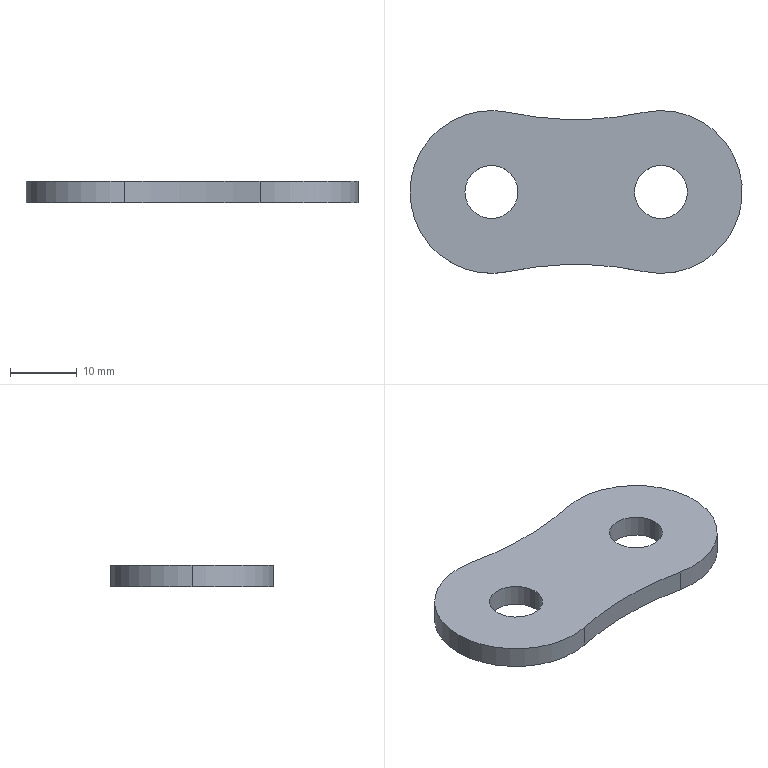Part | STEP file | Outer chain link | 1 solid | 11 faces | box 49.79 x 24.39 x 3.25 mm | volume 3077 mm3 | cylinder 9 | plane 2 | commonest cylinder face diameters 7.94 x4 24.39 x3 97.627 x2
STEP:
#1=CARTESIAN_POINT('',(0.,0.,0.));
#2=DIRECTION('',(0.,0.,1.));
#3=DIRECTION('',(1.,0.,0.));
#4=AXIS2_PLACEMENT_3D('',#1,#2,#3);
#5=CARTESIAN_POINT('',(16.67,0.,0.));
#6=VERTEX_POINT('',#5);
#7=CARTESIAN_POINT('',(16.67,0.,3.25));
#8=VERTEX_POINT('',#7);
#9=CARTESIAN_POINT('',(16.67,0.,0.));
#10=DIRECTION('',(0.,0.,1.));
#11=VECTOR('',#10,1.);
#12=LINE('',#9,#11);
#13=CARTESIAN_POINT('',(12.7,0.,0.));
#14=DIRECTION('',(0.,0.,1.));
#15=DIRECTION('',(1.,0.,0.));
#16=AXIS2_PLACEMENT_3D('',#13,#14,#15);
#17=CYLINDRICAL_SURFACE('',#16,3.97);
#18=CARTESIAN_POINT('',(6.283,0.));
#19=DIRECTION('',(0.,1.));
#20=VECTOR('',#19,1.);
#21=LINE('',#18,#20);
#22=(GEOMETRIC_REPRESENTATION_CONTEXT(2)PARAMETRIC_REPRESENTATION_CONTEXT()REPRESENTATION_CONTEXT('',''));
#23=DEFINITIONAL_REPRESENTATION('',(#21),#22);
#24=PCURVE('',#17,#23);
#25=CARTESIAN_POINT('',(12.7,0.,0.));
#26=DIRECTION('',(0.,0.,1.));
#27=DIRECTION('',(1.,0.,0.));
#28=AXIS2_PLACEMENT_3D('',#25,#26,#27);
#29=CYLINDRICAL_SURFACE('',#28,3.97);
#30=CARTESIAN_POINT('',(0.,0.));
#31=DIRECTION('',(0.,1.));
#32=VECTOR('',#31,1.);
#33=LINE('',#30,#32);
#34=(GEOMETRIC_REPRESENTATION_CONTEXT(2)PARAMETRIC_REPRESENTATION_CONTEXT()REPRESENTATION_CONTEXT('',''));
#35=DEFINITIONAL_REPRESENTATION('',(#33),#34);
#36=PCURVE('',#29,#35);
#37=SURFACE_CURVE('',#12,(#24,#36),.PCURVE_S1.);
#38=EDGE_CURVE('',#6,#8,#37,.T.);
#39=ORIENTED_EDGE('',*,*,#38,.T.);
#40=CARTESIAN_POINT('',(8.73,0.,3.25));
#41=VERTEX_POINT('',#40);
#42=CARTESIAN_POINT('',(12.7,0.,3.25));
#43=DIRECTION('',(0.,0.,1.));
#44=DIRECTION('',(1.,0.,0.));
#45=AXIS2_PLACEMENT_3D('',#42,#43,#44);
#46=CIRCLE('',#45,3.97);
#47=CARTESIAN_POINT('',(0.,3.25));
#48=DIRECTION('',(1.,0.));
#49=VECTOR('',#48,1.);
#50=LINE('',#47,#49);
#51=(GEOMETRIC_REPRESENTATION_CONTEXT(2)PARAMETRIC_REPRESENTATION_CONTEXT()REPRESENTATION_CONTEXT('',''));
#52=DEFINITIONAL_REPRESENTATION('',(#50),#51);
#53=PCURVE('',#17,#52);
#54=CARTESIAN_POINT('',(-6.35,-29.836,3.25));
#55=DIRECTION('',(0.,0.,1.));
#56=DIRECTION('',(1.,0.,0.));
#57=AXIS2_PLACEMENT_3D('',#54,#55,#56);
#58=PLANE('',#57);
#59=CARTESIAN_POINT('',(19.05,29.836));
#60=DIRECTION('',(1.,0.));
#61=AXIS2_PLACEMENT_2D('',#59,#60);
#62=CIRCLE('',#61,3.97);
#63=(GEOMETRIC_REPRESENTATION_CONTEXT(2)PARAMETRIC_REPRESENTATION_CONTEXT()REPRESENTATION_CONTEXT('',''));
#64=DEFINITIONAL_REPRESENTATION('',(#62),#63);
#65=PCURVE('',#58,#64);
#66=SURFACE_CURVE('',#46,(#53,#65),.PCURVE_S1.);
#67=EDGE_CURVE('',#41,#8,#66,.T.);
#68=ORIENTED_EDGE('',*,*,#67,.F.);
#69=CARTESIAN_POINT('',(8.73,0.,0.));
#70=VERTEX_POINT('',#69);
#71=CARTESIAN_POINT('',(8.73,0.,0.));
#72=DIRECTION('',(0.,0.,1.));
#73=VECTOR('',#72,1.);
#74=LINE('',#71,#73);
#75=CARTESIAN_POINT('',(3.142,0.));
#76=DIRECTION('',(0.,1.));
#77=VECTOR('',#76,1.);
#78=LINE('',#75,#77);
#79=(GEOMETRIC_REPRESENTATION_CONTEXT(2)PARAMETRIC_REPRESENTATION_CONTEXT()REPRESENTATION_CONTEXT('',''));
#80=DEFINITIONAL_REPRESENTATION('',(#78),#79);
#81=PCURVE('',#17,#80);
#82=CARTESIAN_POINT('',(3.142,0.));
#83=DIRECTION('',(0.,1.));
#84=VECTOR('',#83,1.);
#85=LINE('',#82,#84);
#86=(GEOMETRIC_REPRESENTATION_CONTEXT(2)PARAMETRIC_REPRESENTATION_CONTEXT()REPRESENTATION_CONTEXT('',''));
#87=DEFINITIONAL_REPRESENTATION('',(#85),#86);
#88=PCURVE('',#29,#87);
#89=SURFACE_CURVE('',#74,(#81,#88),.PCURVE_S1.);
#90=EDGE_CURVE('',#70,#41,#89,.T.);
#91=ORIENTED_EDGE('',*,*,#90,.F.);
#92=CARTESIAN_POINT('',(12.7,0.,0.));
#93=DIRECTION('',(0.,0.,1.));
#94=DIRECTION('',(1.,0.,0.));
#95=AXIS2_PLACEMENT_3D('',#92,#93,#94);
#96=CIRCLE('',#95,3.97);
#97=CARTESIAN_POINT('',(0.,0.));
#98=DIRECTION('',(1.,0.));
#99=VECTOR('',#98,1.);
#100=LINE('',#97,#99);
#101=(GEOMETRIC_REPRESENTATION_CONTEXT(2)PARAMETRIC_REPRESENTATION_CONTEXT()REPRESENTATION_CONTEXT('',''));
#102=DEFINITIONAL_REPRESENTATION('',(#100),#101);
#103=PCURVE('',#17,#102);
#104=CARTESIAN_POINT('',(-6.35,-29.836,0.));
#105=DIRECTION('',(0.,0.,1.));
#106=DIRECTION('',(1.,0.,0.));
#107=AXIS2_PLACEMENT_3D('',#104,#105,#106);
#108=PLANE('',#107);
#109=CARTESIAN_POINT('',(19.05,29.836));
#110=DIRECTION('',(1.,0.));
#111=AXIS2_PLACEMENT_2D('',#109,#110);
#112=CIRCLE('',#111,3.97);
#113=(GEOMETRIC_REPRESENTATION_CONTEXT(2)PARAMETRIC_REPRESENTATION_CONTEXT()REPRESENTATION_CONTEXT('',''));
#114=DEFINITIONAL_REPRESENTATION('',(#112),#113);
#115=PCURVE('',#108,#114);
#116=SURFACE_CURVE('',#96,(#103,#115),.PCURVE_S1.);
#117=EDGE_CURVE('',#70,#6,#116,.T.);
#118=ORIENTED_EDGE('',*,*,#117,.T.);
#119=EDGE_LOOP('',(#39,#68,#91,#118));
#120=FACE_BOUND('',#119,.F.);
#121=ADVANCED_FACE('',(#120),#17,.F.);
#122=CARTESIAN_POINT('',(-8.73,0.,0.));
#123=VERTEX_POINT('',#122);
#124=CARTESIAN_POINT('',(-8.73,0.,3.25));
#125=VERTEX_POINT('',#124);
#126=CARTESIAN_POINT('',(-8.73,0.,0.));
#127=DIRECTION('',(0.,0.,1.));
#128=VECTOR('',#127,1.);
#129=LINE('',#126,#128);
#130=CARTESIAN_POINT('',(-12.7,0.,0.));
#131=DIRECTION('',(0.,0.,1.));
#132=DIRECTION('',(1.,0.,0.));
#133=AXIS2_PLACEMENT_3D('',#130,#131,#132);
#134=CYLINDRICAL_SURFACE('',#133,3.97);
#135=CARTESIAN_POINT('',(6.283,0.));
#136=DIRECTION('',(0.,1.));
#137=VECTOR('',#136,1.);
#138=LINE('',#135,#137);
#139=(GEOMETRIC_REPRESENTATION_CONTEXT(2)PARAMETRIC_REPRESENTATION_CONTEXT()REPRESENTATION_CONTEXT('',''));
#140=DEFINITIONAL_REPRESENTATION('',(#138),#139);
#141=PCURVE('',#134,#140);
#142=CARTESIAN_POINT('',(-12.7,0.,0.));
#143=DIRECTION('',(0.,0.,1.));
#144=DIRECTION('',(1.,0.,0.));
#145=AXIS2_PLACEMENT_3D('',#142,#143,#144);
#146=CYLINDRICAL_SURFACE('',#145,3.97);
#147=CARTESIAN_POINT('',(0.,0.));
#148=DIRECTION('',(0.,1.));
#149=VECTOR('',#148,1.);
#150=LINE('',#147,#149);
#151=(GEOMETRIC_REPRESENTATION_CONTEXT(2)PARAMETRIC_REPRESENTATION_CONTEXT()REPRESENTATION_CONTEXT('',''));
#152=DEFINITIONAL_REPRESENTATION('',(#150),#151);
#153=PCURVE('',#146,#152);
#154=SURFACE_CURVE('',#129,(#141,#153),.PCURVE_S1.);
#155=EDGE_CURVE('',#123,#125,#154,.T.);
#156=ORIENTED_EDGE('',*,*,#155,.T.);
#157=CARTESIAN_POINT('',(-16.67,0.,3.25));
#158=VERTEX_POINT('',#157);
#159=CARTESIAN_POINT('',(-12.7,0.,3.25));
#160=DIRECTION('',(0.,0.,1.));
#161=DIRECTION('',(1.,0.,0.));
#162=AXIS2_PLACEMENT_3D('',#159,#160,#161);
#163=CIRCLE('',#162,3.97);
#164=CARTESIAN_POINT('',(0.,3.25));
#165=DIRECTION('',(1.,0.));
#166=VECTOR('',#165,1.);
#167=LINE('',#164,#166);
#168=(GEOMETRIC_REPRESENTATION_CONTEXT(2)PARAMETRIC_REPRESENTATION_CONTEXT()REPRESENTATION_CONTEXT('',''));
#169=DEFINITIONAL_REPRESENTATION('',(#167),#168);
#170=PCURVE('',#134,#169);
#171=CARTESIAN_POINT('',(-6.35,29.836));
#172=DIRECTION('',(1.,0.));
#173=AXIS2_PLACEMENT_2D('',#171,#172);
#174=CIRCLE('',#173,3.97);
#175=(GEOMETRIC_REPRESENTATION_CONTEXT(2)PARAMETRIC_REPRESENTATION_CONTEXT()REPRESENTATION_CONTEXT('',''));
#176=DEFINITIONAL_REPRESENTATION('',(#174),#175);
#177=PCURVE('',#58,#176);
#178=SURFACE_CURVE('',#163,(#170,#177),.PCURVE_S1.);
#179=EDGE_CURVE('',#158,#125,#178,.T.);
#180=ORIENTED_EDGE('',*,*,#179,.F.);
#181=CARTESIAN_POINT('',(-16.67,0.,0.));
#182=VERTEX_POINT('',#181);
#183=CARTESIAN_POINT('',(-16.67,0.,0.));
#184=DIRECTION('',(0.,0.,1.));
#185=VECTOR('',#184,1.);
#186=LINE('',#183,#185);
#187=CARTESIAN_POINT('',(3.142,0.));
#188=DIRECTION('',(0.,1.));
#189=VECTOR('',#188,1.);
#190=LINE('',#187,#189);
#191=(GEOMETRIC_REPRESENTATION_CONTEXT(2)PARAMETRIC_REPRESENTATION_CONTEXT()REPRESENTATION_CONTEXT('',''));
#192=DEFINITIONAL_REPRESENTATION('',(#190),#191);
#193=PCURVE('',#134,#192);
#194=CARTESIAN_POINT('',(3.142,0.));
#195=DIRECTION('',(0.,1.));
#196=VECTOR('',#195,1.);
#197=LINE('',#194,#196);
#198=(GEOMETRIC_REPRESENTATION_CONTEXT(2)PARAMETRIC_REPRESENTATION_CONTEXT()REPRESENTATION_CONTEXT('',''));
#199=DEFINITIONAL_REPRESENTATION('',(#197),#198);
#200=PCURVE('',#146,#199);
#201=SURFACE_CURVE('',#186,(#193,#200),.PCURVE_S1.);
#202=EDGE_CURVE('',#182,#158,#201,.T.);
#203=ORIENTED_EDGE('',*,*,#202,.F.);
#204=CARTESIAN_POINT('',(-12.7,0.,0.));
#205=DIRECTION('',(0.,0.,1.));
#206=DIRECTION('',(1.,0.,0.));
#207=AXIS2_PLACEMENT_3D('',#204,#205,#206);
#208=CIRCLE('',#207,3.97);
#209=CARTESIAN_POINT('',(0.,0.));
#210=DIRECTION('',(1.,0.));
#211=VECTOR('',#210,1.);
#212=LINE('',#209,#211);
#213=(GEOMETRIC_REPRESENTATION_CONTEXT(2)PARAMETRIC_REPRESENTATION_CONTEXT()REPRESENTATION_CONTEXT('',''));
#214=DEFINITIONAL_REPRESENTATION('',(#212),#213);
#215=PCURVE('',#134,#214);
#216=CARTESIAN_POINT('',(-6.35,29.836));
#217=DIRECTION('',(1.,0.));
#218=AXIS2_PLACEMENT_2D('',#216,#217);
#219=CIRCLE('',#218,3.97);
#220=(GEOMETRIC_REPRESENTATION_CONTEXT(2)PARAMETRIC_REPRESENTATION_CONTEXT()REPRESENTATION_CONTEXT('',''));
#221=DEFINITIONAL_REPRESENTATION('',(#219),#220);
#222=PCURVE('',#108,#221);
#223=SURFACE_CURVE('',#208,(#215,#222),.PCURVE_S1.);
#224=EDGE_CURVE('',#182,#123,#223,.T.);
#225=ORIENTED_EDGE('',*,*,#224,.T.);
#226=EDGE_LOOP('',(#156,#180,#203,#225));
#227=FACE_BOUND('',#226,.F.);
#228=ADVANCED_FACE('',(#227),#134,.F.);
#229=CARTESIAN_POINT('',(-24.895,0.,3.25));
#230=VERTEX_POINT('',#229);
#231=CARTESIAN_POINT('',(-10.161,-11.928,3.25));
#232=VERTEX_POINT('',#231);
#233=CARTESIAN_POINT('',(-12.7,0.,3.25));
#234=DIRECTION('',(0.,0.,1.));
#235=DIRECTION('',(1.,0.,0.));
#236=AXIS2_PLACEMENT_3D('',#233,#234,#235);
#237=CIRCLE('',#236,12.195);
#238=CARTESIAN_POINT('',(-12.7,0.,3.25));
#239=DIRECTION('',(0.,0.,-1.));
#240=DIRECTION('',(-1.,0.,0.));
#241=AXIS2_PLACEMENT_3D('',#238,#239,#240);
#242=CYLINDRICAL_SURFACE('',#241,12.195);
#243=CARTESIAN_POINT('',(9.425,0.));
#244=DIRECTION('',(-1.,0.));
#245=VECTOR('',#244,1.);
#246=LINE('',#243,#245);
#247=(GEOMETRIC_REPRESENTATION_CONTEXT(2)PARAMETRIC_REPRESENTATION_CONTEXT()REPRESENTATION_CONTEXT('',''));
#248=DEFINITIONAL_REPRESENTATION('',(#246),#247);
#249=PCURVE('',#242,#248);
#250=CARTESIAN_POINT('',(-6.35,29.836));
#251=DIRECTION('',(1.,0.));
#252=AXIS2_PLACEMENT_2D('',#250,#251);
#253=CIRCLE('',#252,12.195);
#254=(GEOMETRIC_REPRESENTATION_CONTEXT(2)PARAMETRIC_REPRESENTATION_CONTEXT()REPRESENTATION_CONTEXT('',''));
#255=DEFINITIONAL_REPRESENTATION('',(#253),#254);
#256=PCURVE('',#58,#255);
#257=SURFACE_CURVE('',#237,(#249,#256),.PCURVE_S1.);
#258=EDGE_CURVE('',#230,#232,#257,.T.);
#259=ORIENTED_EDGE('',*,*,#258,.F.);
#260=CARTESIAN_POINT('',(-24.895,0.,0.));
#261=VERTEX_POINT('',#260);
#262=CARTESIAN_POINT('',(-24.895,0.,3.25));
#263=DIRECTION('',(0.,0.,-1.));
#264=VECTOR('',#263,1.);
#265=LINE('',#262,#264);
#266=CARTESIAN_POINT('',(6.283,0.));
#267=DIRECTION('',(0.,1.));
#268=VECTOR('',#267,1.);
#269=LINE('',#266,#268);
#270=(GEOMETRIC_REPRESENTATION_CONTEXT(2)PARAMETRIC_REPRESENTATION_CONTEXT()REPRESENTATION_CONTEXT('',''));
#271=DEFINITIONAL_REPRESENTATION('',(#269),#270);
#272=PCURVE('',#242,#271);
#273=CARTESIAN_POINT('',(-12.7,0.,3.25));
#274=DIRECTION('',(0.,0.,-1.));
#275=DIRECTION('',(-1.,0.,0.));
#276=AXIS2_PLACEMENT_3D('',#273,#274,#275);
#277=CYLINDRICAL_SURFACE('',#276,12.195);
#278=CARTESIAN_POINT('',(0.,0.));
#279=DIRECTION('',(0.,1.));
#280=VECTOR('',#279,1.);
#281=LINE('',#278,#280);
#282=(GEOMETRIC_REPRESENTATION_CONTEXT(2)PARAMETRIC_REPRESENTATION_CONTEXT()REPRESENTATION_CONTEXT('',''));
#283=DEFINITIONAL_REPRESENTATION('',(#281),#282);
#284=PCURVE('',#277,#283);
#285=SURFACE_CURVE('',#265,(#272,#284),.PCURVE_S1.);
#286=EDGE_CURVE('',#230,#261,#285,.T.);
#287=ORIENTED_EDGE('',*,*,#286,.T.);
#288=CARTESIAN_POINT('',(-10.161,-11.928,0.));
#289=VERTEX_POINT('',#288);
#290=CARTESIAN_POINT('',(-12.7,0.,0.));
#291=DIRECTION('',(0.,0.,1.));
#292=DIRECTION('',(1.,0.,0.));
#293=AXIS2_PLACEMENT_3D('',#290,#291,#292);
#294=CIRCLE('',#293,12.195);
#295=CARTESIAN_POINT('',(9.425,3.25));
#296=DIRECTION('',(-1.,0.));
#297=VECTOR('',#296,1.);
#298=LINE('',#295,#297);
#299=(GEOMETRIC_REPRESENTATION_CONTEXT(2)PARAMETRIC_REPRESENTATION_CONTEXT()REPRESENTATION_CONTEXT('',''));
#300=DEFINITIONAL_REPRESENTATION('',(#298),#299);
#301=PCURVE('',#242,#300);
#302=CARTESIAN_POINT('',(-6.35,29.836));
#303=DIRECTION('',(1.,0.));
#304=AXIS2_PLACEMENT_2D('',#302,#303);
#305=CIRCLE('',#304,12.195);
#306=(GEOMETRIC_REPRESENTATION_CONTEXT(2)PARAMETRIC_REPRESENTATION_CONTEXT()REPRESENTATION_CONTEXT('',''));
#307=DEFINITIONAL_REPRESENTATION('',(#305),#306);
#308=PCURVE('',#108,#307);
#309=SURFACE_CURVE('',#294,(#301,#308),.PCURVE_S1.);
#310=EDGE_CURVE('',#261,#289,#309,.T.);
#311=ORIENTED_EDGE('',*,*,#310,.T.);
#312=CARTESIAN_POINT('',(-10.161,-11.928,3.25));
#313=DIRECTION('',(0.,0.,-1.));
#314=VECTOR('',#313,1.);
#315=LINE('',#312,#314);
#316=CARTESIAN_POINT('',(4.503,0.));
#317=DIRECTION('',(0.,1.));
#318=VECTOR('',#317,1.);
#319=LINE('',#316,#318);
#320=(GEOMETRIC_REPRESENTATION_CONTEXT(2)PARAMETRIC_REPRESENTATION_CONTEXT()REPRESENTATION_CONTEXT('',''));
#321=DEFINITIONAL_REPRESENTATION('',(#319),#320);
#322=PCURVE('',#242,#321);
#323=CARTESIAN_POINT('',(0.,-59.672,3.25));
#324=DIRECTION('',(0.,0.,-1.));
#325=DIRECTION('',(-1.,0.,0.));
#326=AXIS2_PLACEMENT_3D('',#323,#324,#325);
#327=CYLINDRICAL_SURFACE('',#326,48.814);
#328=CARTESIAN_POINT('',(1.361,0.));
#329=DIRECTION('',(0.,1.));
#330=VECTOR('',#329,1.);
#331=LINE('',#328,#330);
#332=(GEOMETRIC_REPRESENTATION_CONTEXT(2)PARAMETRIC_REPRESENTATION_CONTEXT()REPRESENTATION_CONTEXT('',''));
#333=DEFINITIONAL_REPRESENTATION('',(#331),#332);
#334=PCURVE('',#327,#333);
#335=SURFACE_CURVE('',#315,(#322,#334),.PCURVE_S1.);
#336=EDGE_CURVE('',#232,#289,#335,.T.);
#337=ORIENTED_EDGE('',*,*,#336,.F.);
#338=EDGE_LOOP('',(#259,#287,#311,#337));
#339=FACE_BOUND('',#338,.T.);
#340=ADVANCED_FACE('',(#339),#242,.T.);
#341=ORIENTED_EDGE('',*,*,#336,.F.);
#342=CARTESIAN_POINT('',(10.161,-11.928,3.25));
#343=VERTEX_POINT('',#342);
#344=CARTESIAN_POINT('',(0.,-59.672,3.25));
#345=DIRECTION('',(0.,0.,-1.));
#346=DIRECTION('',(1.,0.,0.));
#347=AXIS2_PLACEMENT_3D('',#344,#345,#346);
#348=CIRCLE('',#347,48.814);
#349=CARTESIAN_POINT('',(-3.142,0.));
#350=DIRECTION('',(1.,0.));
#351=VECTOR('',#350,1.);
#352=LINE('',#349,#351);
#353=(GEOMETRIC_REPRESENTATION_CONTEXT(2)PARAMETRIC_REPRESENTATION_CONTEXT()REPRESENTATION_CONTEXT('',''));
#354=DEFINITIONAL_REPRESENTATION('',(#352),#353);
#355=PCURVE('',#327,#354);
#356=CARTESIAN_POINT('',(55.164,-29.836));
#357=CARTESIAN_POINT('',(55.164,-114.384));
#358=CARTESIAN_POINT('',(-18.057,-72.11));
#359=CARTESIAN_POINT('',(-91.277,-29.836));
#360=CARTESIAN_POINT('',(-18.057,12.438));
#361=CARTESIAN_POINT('',(55.164,54.712));
#362=CARTESIAN_POINT('',(55.164,-29.836));
#363=(BOUNDED_CURVE()B_SPLINE_CURVE(2,(#356,#357,#358,#359,#360,#361,#362),.UNSPECIFIED.,.T.,.F.)B_SPLINE_CURVE_WITH_KNOTS((1,2,2,2,2,1),(-2.094,0.,2.094,4.189,6.283,8.378),.UNSPECIFIED.)CURVE()GEOMETRIC_REPRESENTATION_ITEM()RATIONAL_B_SPLINE_CURVE((1.,0.5,1.,0.5,1.,0.5,1.))REPRESENTATION_ITEM(''));
#364=(GEOMETRIC_REPRESENTATION_CONTEXT(2)PARAMETRIC_REPRESENTATION_CONTEXT()REPRESENTATION_CONTEXT('',''));
#365=DEFINITIONAL_REPRESENTATION('',(#363),#364);
#366=PCURVE('',#58,#365);
#367=SURFACE_CURVE('',#348,(#355,#366),.PCURVE_S1.);
#368=EDGE_CURVE('',#232,#343,#367,.T.);
#369=ORIENTED_EDGE('',*,*,#368,.T.);
#370=CARTESIAN_POINT('',(10.161,-11.928,0.));
#371=VERTEX_POINT('',#370);
#372=CARTESIAN_POINT('',(10.161,-11.928,3.25));
#373=DIRECTION('',(0.,0.,-1.));
#374=VECTOR('',#373,1.);
#375=LINE('',#372,#374);
#376=CARTESIAN_POINT('',(1.78,0.));
#377=DIRECTION('',(0.,1.));
#378=VECTOR('',#377,1.);
#379=LINE('',#376,#378);
#380=(GEOMETRIC_REPRESENTATION_CONTEXT(2)PARAMETRIC_REPRESENTATION_CONTEXT()REPRESENTATION_CONTEXT('',''));
#381=DEFINITIONAL_REPRESENTATION('',(#379),#380);
#382=PCURVE('',#327,#381);
#383=CARTESIAN_POINT('',(12.7,0.,3.25));
#384=DIRECTION('',(0.,0.,-1.));
#385=DIRECTION('',(-1.,0.,0.));
#386=AXIS2_PLACEMENT_3D('',#383,#384,#385);
#387=CYLINDRICAL_SURFACE('',#386,12.195);
#388=CARTESIAN_POINT('',(4.922,0.));
#389=DIRECTION('',(0.,1.));
#390=VECTOR('',#389,1.);
#391=LINE('',#388,#390);
#392=(GEOMETRIC_REPRESENTATION_CONTEXT(2)PARAMETRIC_REPRESENTATION_CONTEXT()REPRESENTATION_CONTEXT('',''));
#393=DEFINITIONAL_REPRESENTATION('',(#391),#392);
#394=PCURVE('',#387,#393);
#395=SURFACE_CURVE('',#375,(#382,#394),.PCURVE_S1.);
#396=EDGE_CURVE('',#343,#371,#395,.T.);
#397=ORIENTED_EDGE('',*,*,#396,.T.);
#398=CARTESIAN_POINT('',(0.,-59.672,0.));
#399=DIRECTION('',(0.,0.,-1.));
#400=DIRECTION('',(1.,0.,0.));
#401=AXIS2_PLACEMENT_3D('',#398,#399,#400);
#402=CIRCLE('',#401,48.814);
#403=CARTESIAN_POINT('',(-3.142,3.25));
#404=DIRECTION('',(1.,0.));
#405=VECTOR('',#404,1.);
#406=LINE('',#403,#405);
#407=(GEOMETRIC_REPRESENTATION_CONTEXT(2)PARAMETRIC_REPRESENTATION_CONTEXT()REPRESENTATION_CONTEXT('',''));
#408=DEFINITIONAL_REPRESENTATION('',(#406),#407);
#409=PCURVE('',#327,#408);
#410=CARTESIAN_POINT('',(55.164,-29.836));
#411=CARTESIAN_POINT('',(55.164,-114.384));
#412=CARTESIAN_POINT('',(-18.057,-72.11));
#413=CARTESIAN_POINT('',(-91.277,-29.836));
#414=CARTESIAN_POINT('',(-18.057,12.438));
#415=CARTESIAN_POINT('',(55.164,54.712));
#416=CARTESIAN_POINT('',(55.164,-29.836));
#417=(BOUNDED_CURVE()B_SPLINE_CURVE(2,(#410,#411,#412,#413,#414,#415,#416),.UNSPECIFIED.,.T.,.F.)B_SPLINE_CURVE_WITH_KNOTS((1,2,2,2,2,1),(-2.094,0.,2.094,4.189,6.283,8.378),.UNSPECIFIED.)CURVE()GEOMETRIC_REPRESENTATION_ITEM()RATIONAL_B_SPLINE_CURVE((1.,0.5,1.,0.5,1.,0.5,1.))REPRESENTATION_ITEM(''));
#418=(GEOMETRIC_REPRESENTATION_CONTEXT(2)PARAMETRIC_REPRESENTATION_CONTEXT()REPRESENTATION_CONTEXT('',''));
#419=DEFINITIONAL_REPRESENTATION('',(#417),#418);
#420=PCURVE('',#108,#419);
#421=SURFACE_CURVE('',#402,(#409,#420),.PCURVE_S1.);
#422=EDGE_CURVE('',#289,#371,#421,.T.);
#423=ORIENTED_EDGE('',*,*,#422,.F.);
#424=EDGE_LOOP('',(#341,#369,#397,#423));
#425=FACE_BOUND('',#424,.F.);
#426=ADVANCED_FACE('',(#425),#327,.F.);
#427=CARTESIAN_POINT('',(10.161,11.928,0.));
#428=VERTEX_POINT('',#427);
#429=CARTESIAN_POINT('',(12.7,0.,0.));
#430=DIRECTION('',(0.,0.,1.));
#431=DIRECTION('',(1.,0.,0.));
#432=AXIS2_PLACEMENT_3D('',#429,#430,#431);
#433=CIRCLE('',#432,12.195);
#434=CARTESIAN_POINT('',(9.425,3.25));
#435=DIRECTION('',(-1.,0.));
#436=VECTOR('',#435,1.);
#437=LINE('',#434,#436);
#438=(GEOMETRIC_REPRESENTATION_CONTEXT(2)PARAMETRIC_REPRESENTATION_CONTEXT()REPRESENTATION_CONTEXT('',''));
#439=DEFINITIONAL_REPRESENTATION('',(#437),#438);
#440=PCURVE('',#387,#439);
#441=CARTESIAN_POINT('',(19.05,29.836));
#442=DIRECTION('',(1.,0.));
#443=AXIS2_PLACEMENT_2D('',#441,#442);
#444=CIRCLE('',#443,12.195);
#445=(GEOMETRIC_REPRESENTATION_CONTEXT(2)PARAMETRIC_REPRESENTATION_CONTEXT()REPRESENTATION_CONTEXT('',''));
#446=DEFINITIONAL_REPRESENTATION('',(#444),#445);
#447=PCURVE('',#108,#446);
#448=SURFACE_CURVE('',#433,(#440,#447),.PCURVE_S1.);
#449=EDGE_CURVE('',#371,#428,#448,.T.);
#450=ORIENTED_EDGE('',*,*,#449,.T.);
#451=CARTESIAN_POINT('',(10.161,11.928,3.25));
#452=VERTEX_POINT('',#451);
#453=CARTESIAN_POINT('',(10.161,11.928,3.25));
#454=DIRECTION('',(0.,0.,-1.));
#455=VECTOR('',#454,1.);
#456=LINE('',#453,#455);
#457=CARTESIAN_POINT('',(1.361,0.));
#458=DIRECTION('',(0.,1.));
#459=VECTOR('',#458,1.);
#460=LINE('',#457,#459);
#461=(GEOMETRIC_REPRESENTATION_CONTEXT(2)PARAMETRIC_REPRESENTATION_CONTEXT()REPRESENTATION_CONTEXT('',''));
#462=DEFINITIONAL_REPRESENTATION('',(#460),#461);
#463=PCURVE('',#387,#462);
#464=CARTESIAN_POINT('',(0.,59.672,3.25));
#465=DIRECTION('',(0.,0.,-1.));
#466=DIRECTION('',(-1.,0.,0.));
#467=AXIS2_PLACEMENT_3D('',#464,#465,#466);
#468=CYLINDRICAL_SURFACE('',#467,48.814);
#469=CARTESIAN_POINT('',(4.503,0.));
#470=DIRECTION('',(0.,1.));
#471=VECTOR('',#470,1.);
#472=LINE('',#469,#471);
#473=(GEOMETRIC_REPRESENTATION_CONTEXT(2)PARAMETRIC_REPRESENTATION_CONTEXT()REPRESENTATION_CONTEXT('',''));
#474=DEFINITIONAL_REPRESENTATION('',(#472),#473);
#475=PCURVE('',#468,#474);
#476=SURFACE_CURVE('',#456,(#463,#475),.PCURVE_S1.);
#477=EDGE_CURVE('',#452,#428,#476,.T.);
#478=ORIENTED_EDGE('',*,*,#477,.F.);
#479=CARTESIAN_POINT('',(12.7,0.,3.25));
#480=DIRECTION('',(0.,0.,1.));
#481=DIRECTION('',(1.,0.,0.));
#482=AXIS2_PLACEMENT_3D('',#479,#480,#481);
#483=CIRCLE('',#482,12.195);
#484=CARTESIAN_POINT('',(9.425,0.));
#485=DIRECTION('',(-1.,0.));
#486=VECTOR('',#485,1.);
#487=LINE('',#484,#486);
#488=(GEOMETRIC_REPRESENTATION_CONTEXT(2)PARAMETRIC_REPRESENTATION_CONTEXT()REPRESENTATION_CONTEXT('',''));
#489=DEFINITIONAL_REPRESENTATION('',(#487),#488);
#490=PCURVE('',#387,#489);
#491=CARTESIAN_POINT('',(19.05,29.836));
#492=DIRECTION('',(1.,0.));
#493=AXIS2_PLACEMENT_2D('',#491,#492);
#494=CIRCLE('',#493,12.195);
#495=(GEOMETRIC_REPRESENTATION_CONTEXT(2)PARAMETRIC_REPRESENTATION_CONTEXT()REPRESENTATION_CONTEXT('',''));
#496=DEFINITIONAL_REPRESENTATION('',(#494),#495);
#497=PCURVE('',#58,#496);
#498=SURFACE_CURVE('',#483,(#490,#497),.PCURVE_S1.);
#499=EDGE_CURVE('',#343,#452,#498,.T.);
#500=ORIENTED_EDGE('',*,*,#499,.F.);
#501=ORIENTED_EDGE('',*,*,#396,.T.);
#502=EDGE_LOOP('',(#450,#478,#500,#501));
#503=FACE_BOUND('',#502,.T.);
#504=ADVANCED_FACE('',(#503),#387,.T.);
#505=ORIENTED_EDGE('',*,*,#477,.F.);
#506=CARTESIAN_POINT('',(-10.161,11.928,3.25));
#507=VERTEX_POINT('',#506);
#508=CARTESIAN_POINT('',(0.,59.672,3.25));
#509=DIRECTION('',(0.,0.,-1.));
#510=DIRECTION('',(1.,0.,0.));
#511=AXIS2_PLACEMENT_3D('',#508,#509,#510);
#512=CIRCLE('',#511,48.814);
#513=CARTESIAN_POINT('',(3.142,0.));
#514=DIRECTION('',(1.,0.));
#515=VECTOR('',#514,1.);
#516=LINE('',#513,#515);
#517=(GEOMETRIC_REPRESENTATION_CONTEXT(2)PARAMETRIC_REPRESENTATION_CONTEXT()REPRESENTATION_CONTEXT('',''));
#518=DEFINITIONAL_REPRESENTATION('',(#516),#517);
#519=PCURVE('',#468,#518);
#520=CARTESIAN_POINT('',(55.164,89.508));
#521=CARTESIAN_POINT('',(55.164,4.96));
#522=CARTESIAN_POINT('',(-18.057,47.234));
#523=CARTESIAN_POINT('',(-91.277,89.508));
#524=CARTESIAN_POINT('',(-18.057,131.782));
#525=CARTESIAN_POINT('',(55.164,174.056));
#526=CARTESIAN_POINT('',(55.164,89.508));
#527=(BOUNDED_CURVE()B_SPLINE_CURVE(2,(#520,#521,#522,#523,#524,#525,#526),.UNSPECIFIED.,.T.,.F.)B_SPLINE_CURVE_WITH_KNOTS((1,2,2,2,2,1),(-2.094,0.,2.094,4.189,6.283,8.378),.UNSPECIFIED.)CURVE()GEOMETRIC_REPRESENTATION_ITEM()RATIONAL_B_SPLINE_CURVE((1.,0.5,1.,0.5,1.,0.5,1.))REPRESENTATION_ITEM(''));
#528=(GEOMETRIC_REPRESENTATION_CONTEXT(2)PARAMETRIC_REPRESENTATION_CONTEXT()REPRESENTATION_CONTEXT('',''));
#529=DEFINITIONAL_REPRESENTATION('',(#527),#528);
#530=PCURVE('',#58,#529);
#531=SURFACE_CURVE('',#512,(#519,#530),.PCURVE_S1.);
#532=EDGE_CURVE('',#452,#507,#531,.T.);
#533=ORIENTED_EDGE('',*,*,#532,.T.);
#534=CARTESIAN_POINT('',(-10.161,11.928,0.));
#535=VERTEX_POINT('',#534);
#536=CARTESIAN_POINT('',(-10.161,11.928,3.25));
#537=DIRECTION('',(0.,0.,-1.));
#538=VECTOR('',#537,1.);
#539=LINE('',#536,#538);
#540=CARTESIAN_POINT('',(4.922,0.));
#541=DIRECTION('',(0.,1.));
#542=VECTOR('',#541,1.);
#543=LINE('',#540,#542);
#544=(GEOMETRIC_REPRESENTATION_CONTEXT(2)PARAMETRIC_REPRESENTATION_CONTEXT()REPRESENTATION_CONTEXT('',''));
#545=DEFINITIONAL_REPRESENTATION('',(#543),#544);
#546=PCURVE('',#468,#545);
#547=CARTESIAN_POINT('',(1.78,0.));
#548=DIRECTION('',(0.,1.));
#549=VECTOR('',#548,1.);
#550=LINE('',#547,#549);
#551=(GEOMETRIC_REPRESENTATION_CONTEXT(2)PARAMETRIC_REPRESENTATION_CONTEXT()REPRESENTATION_CONTEXT('',''));
#552=DEFINITIONAL_REPRESENTATION('',(#550),#551);
#553=PCURVE('',#277,#552);
#554=SURFACE_CURVE('',#539,(#546,#553),.PCURVE_S1.);
#555=EDGE_CURVE('',#507,#535,#554,.T.);
#556=ORIENTED_EDGE('',*,*,#555,.T.);
#557=CARTESIAN_POINT('',(0.,59.672,0.));
#558=DIRECTION('',(0.,0.,-1.));
#559=DIRECTION('',(1.,0.,0.));
#560=AXIS2_PLACEMENT_3D('',#557,#558,#559);
#561=CIRCLE('',#560,48.814);
#562=CARTESIAN_POINT('',(3.142,3.25));
#563=DIRECTION('',(1.,0.));
#564=VECTOR('',#563,1.);
#565=LINE('',#562,#564);
#566=(GEOMETRIC_REPRESENTATION_CONTEXT(2)PARAMETRIC_REPRESENTATION_CONTEXT()REPRESENTATION_CONTEXT('',''));
#567=DEFINITIONAL_REPRESENTATION('',(#565),#566);
#568=PCURVE('',#468,#567);
#569=CARTESIAN_POINT('',(55.164,89.508));
#570=CARTESIAN_POINT('',(55.164,4.96));
#571=CARTESIAN_POINT('',(-18.057,47.234));
#572=CARTESIAN_POINT('',(-91.277,89.508));
#573=CARTESIAN_POINT('',(-18.057,131.782));
#574=CARTESIAN_POINT('',(55.164,174.056));
#575=CARTESIAN_POINT('',(55.164,89.508));
#576=(BOUNDED_CURVE()B_SPLINE_CURVE(2,(#569,#570,#571,#572,#573,#574,#575),.UNSPECIFIED.,.T.,.F.)B_SPLINE_CURVE_WITH_KNOTS((1,2,2,2,2,1),(-2.094,0.,2.094,4.189,6.283,8.378),.UNSPECIFIED.)CURVE()GEOMETRIC_REPRESENTATION_ITEM()RATIONAL_B_SPLINE_CURVE((1.,0.5,1.,0.5,1.,0.5,1.))REPRESENTATION_ITEM(''));
#577=(GEOMETRIC_REPRESENTATION_CONTEXT(2)PARAMETRIC_REPRESENTATION_CONTEXT()REPRESENTATION_CONTEXT('',''));
#578=DEFINITIONAL_REPRESENTATION('',(#576),#577);
#579=PCURVE('',#108,#578);
#580=SURFACE_CURVE('',#561,(#568,#579),.PCURVE_S1.);
#581=EDGE_CURVE('',#428,#535,#580,.T.);
#582=ORIENTED_EDGE('',*,*,#581,.F.);
#583=EDGE_LOOP('',(#505,#533,#556,#582));
#584=FACE_BOUND('',#583,.F.);
#585=ADVANCED_FACE('',(#584),#468,.F.);
#586=ORIENTED_EDGE('',*,*,#286,.F.);
#587=CARTESIAN_POINT('',(-12.7,0.,3.25));
#588=DIRECTION('',(0.,0.,1.));
#589=DIRECTION('',(1.,0.,0.));
#590=AXIS2_PLACEMENT_3D('',#587,#588,#589);
#591=CIRCLE('',#590,12.195);
#592=CARTESIAN_POINT('',(3.142,0.));
#593=DIRECTION('',(-1.,0.));
#594=VECTOR('',#593,1.);
#595=LINE('',#592,#594);
#596=(GEOMETRIC_REPRESENTATION_CONTEXT(2)PARAMETRIC_REPRESENTATION_CONTEXT()REPRESENTATION_CONTEXT('',''));
#597=DEFINITIONAL_REPRESENTATION('',(#595),#596);
#598=PCURVE('',#277,#597);
#599=CARTESIAN_POINT('',(-6.35,29.836));
#600=DIRECTION('',(1.,0.));
#601=AXIS2_PLACEMENT_2D('',#599,#600);
#602=CIRCLE('',#601,12.195);
#603=(GEOMETRIC_REPRESENTATION_CONTEXT(2)PARAMETRIC_REPRESENTATION_CONTEXT()REPRESENTATION_CONTEXT('',''));
#604=DEFINITIONAL_REPRESENTATION('',(#602),#603);
#605=PCURVE('',#58,#604);
#606=SURFACE_CURVE('',#591,(#598,#605),.PCURVE_S1.);
#607=EDGE_CURVE('',#507,#230,#606,.T.);
#608=ORIENTED_EDGE('',*,*,#607,.F.);
#609=ORIENTED_EDGE('',*,*,#555,.T.);
#610=CARTESIAN_POINT('',(-12.7,0.,0.));
#611=DIRECTION('',(0.,0.,1.));
#612=DIRECTION('',(1.,0.,0.));
#613=AXIS2_PLACEMENT_3D('',#610,#611,#612);
#614=CIRCLE('',#613,12.195);
#615=CARTESIAN_POINT('',(3.142,3.25));
#616=DIRECTION('',(-1.,0.));
#617=VECTOR('',#616,1.);
#618=LINE('',#615,#617);
#619=(GEOMETRIC_REPRESENTATION_CONTEXT(2)PARAMETRIC_REPRESENTATION_CONTEXT()REPRESENTATION_CONTEXT('',''));
#620=DEFINITIONAL_REPRESENTATION('',(#618),#619);
#621=PCURVE('',#277,#620);
#622=CARTESIAN_POINT('',(-6.35,29.836));
#623=DIRECTION('',(1.,0.));
#624=AXIS2_PLACEMENT_2D('',#622,#623);
#625=CIRCLE('',#624,12.195);
#626=(GEOMETRIC_REPRESENTATION_CONTEXT(2)PARAMETRIC_REPRESENTATION_CONTEXT()REPRESENTATION_CONTEXT('',''));
#627=DEFINITIONAL_REPRESENTATION('',(#625),#626);
#628=PCURVE('',#108,#627);
#629=SURFACE_CURVE('',#614,(#621,#628),.PCURVE_S1.);
#630=EDGE_CURVE('',#535,#261,#629,.T.);
#631=ORIENTED_EDGE('',*,*,#630,.T.);
#632=EDGE_LOOP('',(#586,#608,#609,#631));
#633=FACE_BOUND('',#632,.T.);
#634=ADVANCED_FACE('',(#633),#277,.T.);
#635=CARTESIAN_POINT('',(12.7,0.,3.25));
#636=DIRECTION('',(0.,0.,1.));
#637=DIRECTION('',(1.,0.,0.));
#638=AXIS2_PLACEMENT_3D('',#635,#636,#637);
#639=CIRCLE('',#638,3.97);
#640=CARTESIAN_POINT('',(19.05,29.836));
#641=DIRECTION('',(1.,0.));
#642=AXIS2_PLACEMENT_2D('',#640,#641);
#643=CIRCLE('',#642,3.97);
#644=(GEOMETRIC_REPRESENTATION_CONTEXT(2)PARAMETRIC_REPRESENTATION_CONTEXT()REPRESENTATION_CONTEXT('',''));
#645=DEFINITIONAL_REPRESENTATION('',(#643),#644);
#646=PCURVE('',#58,#645);
#647=CARTESIAN_POINT('',(0.,3.25));
#648=DIRECTION('',(1.,0.));
#649=VECTOR('',#648,1.);
#650=LINE('',#647,#649);
#651=(GEOMETRIC_REPRESENTATION_CONTEXT(2)PARAMETRIC_REPRESENTATION_CONTEXT()REPRESENTATION_CONTEXT('',''));
#652=DEFINITIONAL_REPRESENTATION('',(#650),#651);
#653=PCURVE('',#29,#652);
#654=SURFACE_CURVE('',#639,(#646,#653),.PCURVE_S1.);
#655=EDGE_CURVE('',#8,#41,#654,.T.);
#656=ORIENTED_EDGE('',*,*,#655,.F.);
#657=ORIENTED_EDGE('',*,*,#67,.F.);
#658=EDGE_LOOP('',(#656,#657));
#659=FACE_BOUND('',#658,.T.);
#660=CARTESIAN_POINT('',(-12.7,0.,3.25));
#661=DIRECTION('',(0.,0.,1.));
#662=DIRECTION('',(1.,0.,0.));
#663=AXIS2_PLACEMENT_3D('',#660,#661,#662);
#664=CIRCLE('',#663,3.97);
#665=CARTESIAN_POINT('',(-6.35,29.836));
#666=DIRECTION('',(1.,0.));
#667=AXIS2_PLACEMENT_2D('',#665,#666);
#668=CIRCLE('',#667,3.97);
#669=(GEOMETRIC_REPRESENTATION_CONTEXT(2)PARAMETRIC_REPRESENTATION_CONTEXT()REPRESENTATION_CONTEXT('',''));
#670=DEFINITIONAL_REPRESENTATION('',(#668),#669);
#671=PCURVE('',#58,#670);
#672=CARTESIAN_POINT('',(0.,3.25));
#673=DIRECTION('',(1.,0.));
#674=VECTOR('',#673,1.);
#675=LINE('',#672,#674);
#676=(GEOMETRIC_REPRESENTATION_CONTEXT(2)PARAMETRIC_REPRESENTATION_CONTEXT()REPRESENTATION_CONTEXT('',''));
#677=DEFINITIONAL_REPRESENTATION('',(#675),#676);
#678=PCURVE('',#146,#677);
#679=SURFACE_CURVE('',#664,(#671,#678),.PCURVE_S1.);
#680=EDGE_CURVE('',#125,#158,#679,.T.);
#681=ORIENTED_EDGE('',*,*,#680,.F.);
#682=ORIENTED_EDGE('',*,*,#179,.F.);
#683=EDGE_LOOP('',(#681,#682));
#684=FACE_BOUND('',#683,.T.);
#685=ORIENTED_EDGE('',*,*,#368,.T.);
#686=ORIENTED_EDGE('',*,*,#499,.T.);
#687=ORIENTED_EDGE('',*,*,#532,.T.);
#688=ORIENTED_EDGE('',*,*,#607,.T.);
#689=ORIENTED_EDGE('',*,*,#258,.T.);
#690=EDGE_LOOP('',(#685,#686,#687,#688,#689));
#691=FACE_BOUND('',#690,.T.);
#692=ADVANCED_FACE('',(#659,#684,#691),#58,.T.);
#693=CARTESIAN_POINT('',(12.7,0.,0.));
#694=DIRECTION('',(0.,0.,1.));
#695=DIRECTION('',(1.,0.,0.));
#696=AXIS2_PLACEMENT_3D('',#693,#694,#695);
#697=CIRCLE('',#696,3.97);
#698=CARTESIAN_POINT('',(19.05,29.836));
#699=DIRECTION('',(1.,0.));
#700=AXIS2_PLACEMENT_2D('',#698,#699);
#701=CIRCLE('',#700,3.97);
#702=(GEOMETRIC_REPRESENTATION_CONTEXT(2)PARAMETRIC_REPRESENTATION_CONTEXT()REPRESENTATION_CONTEXT('',''));
#703=DEFINITIONAL_REPRESENTATION('',(#701),#702);
#704=PCURVE('',#108,#703);
#705=CARTESIAN_POINT('',(0.,0.));
#706=DIRECTION('',(1.,0.));
#707=VECTOR('',#706,1.);
#708=LINE('',#705,#707);
#709=(GEOMETRIC_REPRESENTATION_CONTEXT(2)PARAMETRIC_REPRESENTATION_CONTEXT()REPRESENTATION_CONTEXT('',''));
#710=DEFINITIONAL_REPRESENTATION('',(#708),#709);
#711=PCURVE('',#29,#710);
#712=SURFACE_CURVE('',#697,(#704,#711),.PCURVE_S1.);
#713=EDGE_CURVE('',#6,#70,#712,.T.);
#714=ORIENTED_EDGE('',*,*,#713,.T.);
#715=ORIENTED_EDGE('',*,*,#117,.T.);
#716=EDGE_LOOP('',(#714,#715));
#717=FACE_BOUND('',#716,.T.);
#718=CARTESIAN_POINT('',(-12.7,0.,0.));
#719=DIRECTION('',(0.,0.,1.));
#720=DIRECTION('',(1.,0.,0.));
#721=AXIS2_PLACEMENT_3D('',#718,#719,#720);
#722=CIRCLE('',#721,3.97);
#723=CARTESIAN_POINT('',(-6.35,29.836));
#724=DIRECTION('',(1.,0.));
#725=AXIS2_PLACEMENT_2D('',#723,#724);
#726=CIRCLE('',#725,3.97);
#727=(GEOMETRIC_REPRESENTATION_CONTEXT(2)PARAMETRIC_REPRESENTATION_CONTEXT()REPRESENTATION_CONTEXT('',''));
#728=DEFINITIONAL_REPRESENTATION('',(#726),#727);
#729=PCURVE('',#108,#728);
#730=CARTESIAN_POINT('',(0.,0.));
#731=DIRECTION('',(1.,0.));
#732=VECTOR('',#731,1.);
#733=LINE('',#730,#732);
#734=(GEOMETRIC_REPRESENTATION_CONTEXT(2)PARAMETRIC_REPRESENTATION_CONTEXT()REPRESENTATION_CONTEXT('',''));
#735=DEFINITIONAL_REPRESENTATION('',(#733),#734);
#736=PCURVE('',#146,#735);
#737=SURFACE_CURVE('',#722,(#729,#736),.PCURVE_S1.);
#738=EDGE_CURVE('',#123,#182,#737,.T.);
#739=ORIENTED_EDGE('',*,*,#738,.T.);
#740=ORIENTED_EDGE('',*,*,#224,.T.);
#741=EDGE_LOOP('',(#739,#740));
#742=FACE_BOUND('',#741,.T.);
#743=ORIENTED_EDGE('',*,*,#422,.F.);
#744=ORIENTED_EDGE('',*,*,#310,.F.);
#745=ORIENTED_EDGE('',*,*,#630,.F.);
#746=ORIENTED_EDGE('',*,*,#581,.F.);
#747=ORIENTED_EDGE('',*,*,#449,.F.);
#748=EDGE_LOOP('',(#743,#744,#745,#746,#747));
#749=FACE_BOUND('',#748,.T.);
#750=ADVANCED_FACE('',(#717,#742,#749),#108,.F.);
#751=ORIENTED_EDGE('',*,*,#680,.F.);
#752=ORIENTED_EDGE('',*,*,#155,.F.);
#753=ORIENTED_EDGE('',*,*,#738,.T.);
#754=ORIENTED_EDGE('',*,*,#202,.T.);
#755=EDGE_LOOP('',(#751,#752,#753,#754));
#756=FACE_BOUND('',#755,.F.);
#757=ADVANCED_FACE('',(#756),#146,.F.);
#758=ORIENTED_EDGE('',*,*,#655,.F.);
#759=ORIENTED_EDGE('',*,*,#38,.F.);
#760=ORIENTED_EDGE('',*,*,#713,.T.);
#761=ORIENTED_EDGE('',*,*,#90,.T.);
#762=EDGE_LOOP('',(#758,#759,#760,#761));
#763=FACE_BOUND('',#762,.F.);
#764=ADVANCED_FACE('',(#763),#29,.F.);
#765=CLOSED_SHELL('',(#121,#228,#340,#426,#504,#585,#634,#692,#750,#757,#764));
#766=MANIFOLD_SOLID_BREP('',#765);
#767=(LENGTH_UNIT()NAMED_UNIT(*)SI_UNIT(.MILLI.,.METRE.));
#768=UNCERTAINTY_MEASURE_WITH_UNIT(LENGTH_MEASURE(0.0000001),#767,'','');
#769=(NAMED_UNIT(*)PLANE_ANGLE_UNIT()SI_UNIT($,.RADIAN.));
#770=(NAMED_UNIT(*)SI_UNIT($,.STERADIAN.)SOLID_ANGLE_UNIT());
#771=(GEOMETRIC_REPRESENTATION_CONTEXT(3)GLOBAL_UNCERTAINTY_ASSIGNED_CONTEXT((#768))GLOBAL_UNIT_ASSIGNED_CONTEXT((#767,#769,#770))REPRESENTATION_CONTEXT('',''));
#772=ADVANCED_BREP_SHAPE_REPRESENTATION('',(#4,#766),#771);